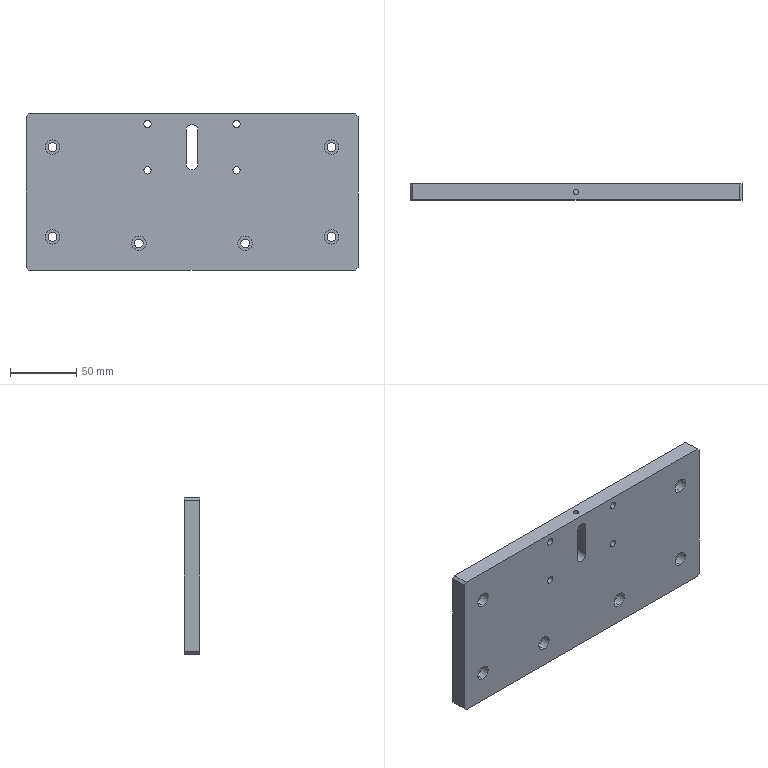Part | SolidWorks | features HoleWzd 4, Chamfer 1, Extrusion 1 | 1 solid | 67 faces | box 250 x 12 x 117.5 mm | volume 341494 mm3 | cylinder 45 | plane 22 | commonest cylinder face diameters 6.6 x12 11 x12 5.5 x8 10 x8 9 x3 4.2 x2